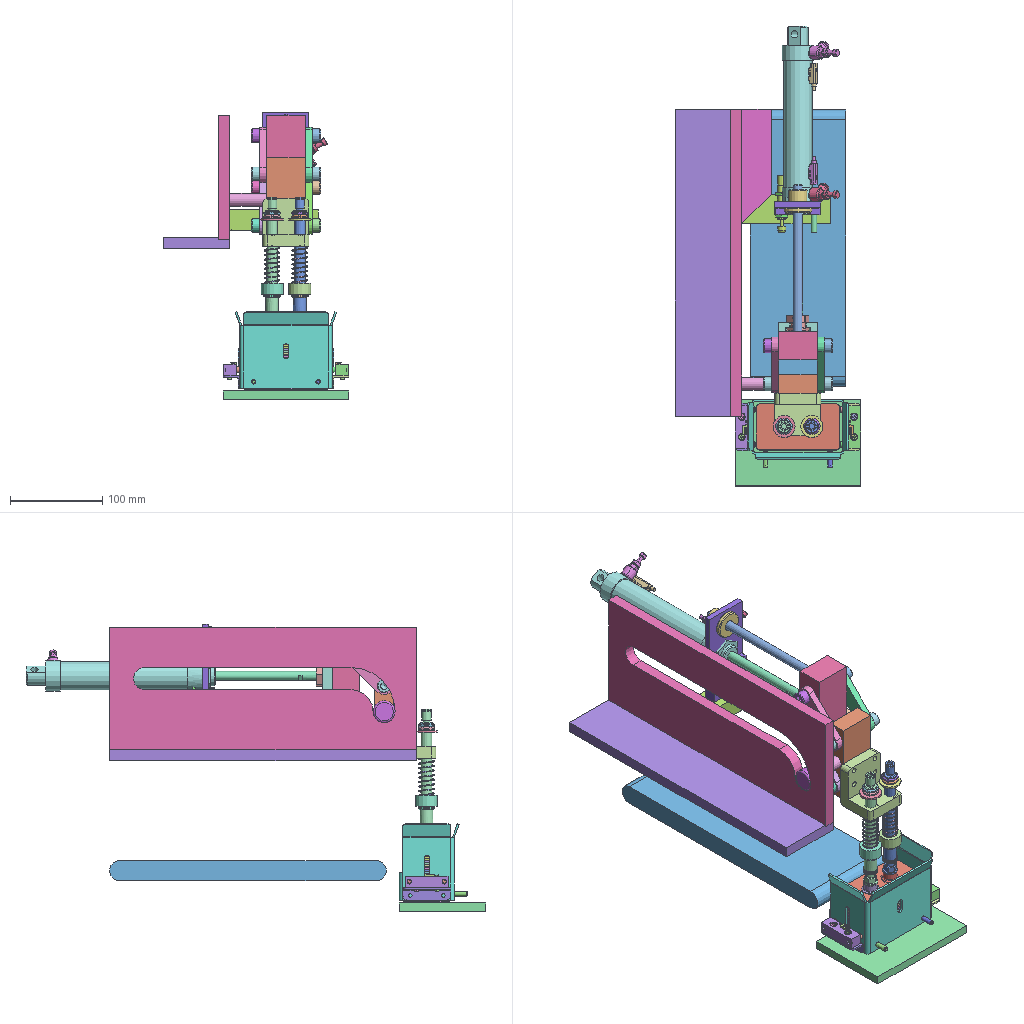Assembly | NX | 102 different items | 102 placed | box 201 x 499 x 312 mm
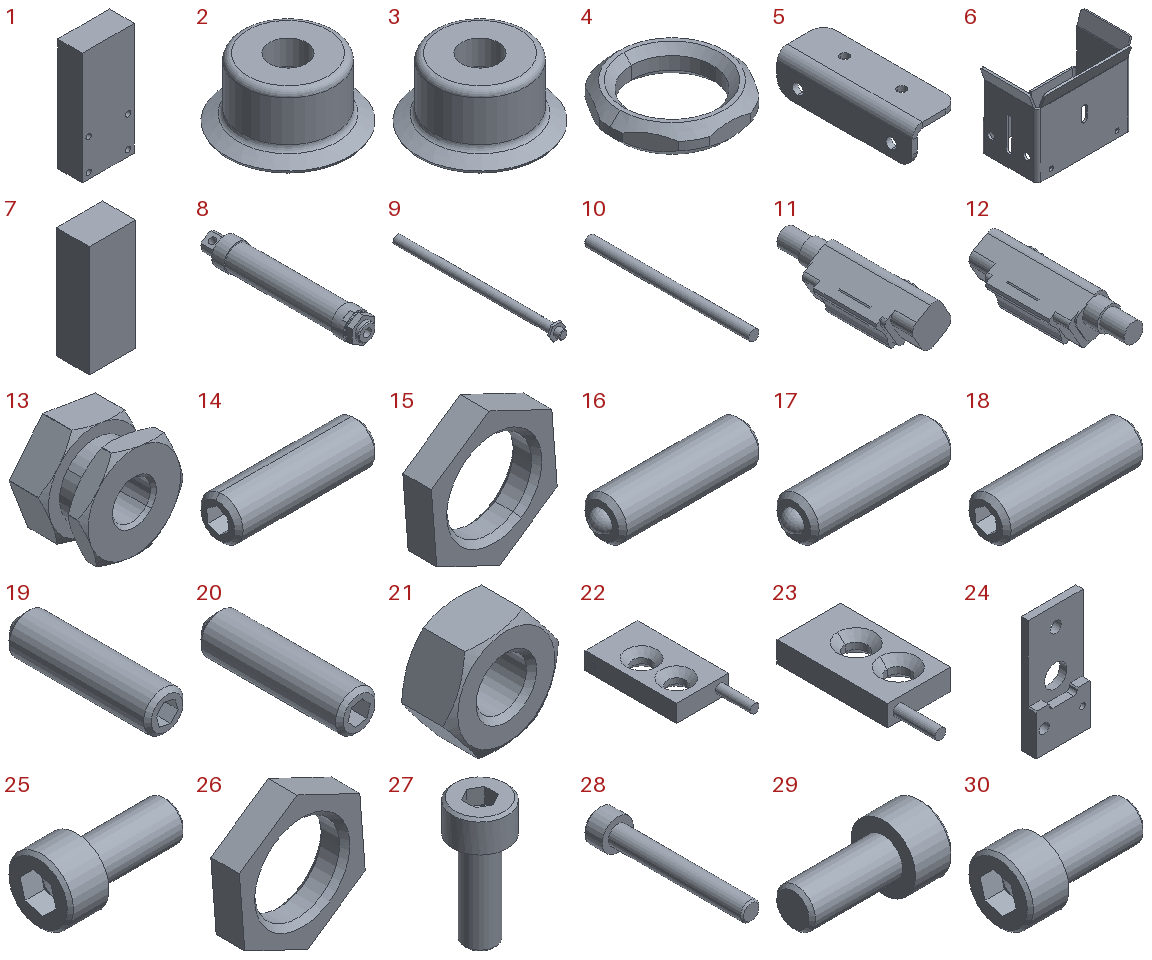Parts list (item | quantity | size | volume | features):
1 | x1 | 42 x 20 x 91 mm | 75332 mm3 | features M5 螺纹孔1 2
2 | x1 | 20 x 20 x 10 mm | 1200 mm3 | features 输入1 2
3 | x1 | 20 x 20 x 10 mm | 1200 mm3 | features 输入1 2
4 | x1 | 18 x 17 x 4 mm | 405.702 mm3 | features 输入1 2
5 | x1 | 18 x 52 x 14 mm | 2859 mm3 | features 镜向1 2
6 | x1 | 110.019 x 65.01 x 82.801 mm | 38324 mm3 | features M5 螺纹孔1 2
7 | x1 | 42 x 30 x 101 mm | 127260 mm3 | features M5 螺纹孔1 2
8 | x1 | 34 x 205 x 34 mm | 131750 mm3 | features WGN01-25-100-Y-2-001 2
9 | x1 | 19.589 x 203 x 17.595 mm | 16333 mm3 | features WGN01-25-100-Y-2-002 2
10 | x1 | 10 x 159.55 x 10 mm | 12516 mm3 | features WGN01-25-100-Y-2-002 2
11 | x1 | 10.179 x 30 x 9.481 mm | 1272 mm3 | features WGN01-25-100-Y-2-003 2
12 | x1 | 10.179 x 30 x 9.481 mm | 1272 mm3 | features WGN01-25-100-Y-2-003 2
13 | x1 | 23.903 x 16.5 x 22.65 mm | 4391 mm3 | features WHC31-M10-1_25-L8.SLDPRT 2
14 | x1 | 21.3 x 6 x 6 mm | 545.053 mm3 | features _ZAH01-M6 2
15 | x1 | 13.228 x 3 x 14.621 mm | 223.149 mm3 | features CONE_1 2
16 | x1 | 21.3 x 6 x 6 mm | 545.05 mm3 | features _ZAH01-M6 2
17 | x1 | 21.3 x 6 x 6 mm | 545.05 mm3 | features _ZAH01-M6 2
18 | x1 | 21.3 x 6 x 6 mm | 545.05 mm3 | features _ZAH01-M6 2
19 | x1 | 5 x 19.3 x 5 mm | 344.732 mm3 | features _ZAH04-M5 2
20 | x1 | 5 x 19.3 x 5 mm | 344.732 mm3 | features _ZAH04-M5 2
21 | x1 | 11.434 x 5.2 x 10.707 mm | 339.24 mm3 | features 倒角1 2
22 | x1 | 6.1 x 14.5 x 2 mm | 107.405 mm3 | features 倒角1 2
23 | x1 | 6.1 x 14.5 x 2 mm | 107.405 mm3 | features 倒角1 2
24 | x1 | 50 x 13.5 x 106 mm | 42427 mm3 | features 倒角2 2
25 | x1 | 30 x 15 x 15 mm | 2656 mm3 | features 切除-拉伸1 2
26 | x1 | 13.228 x 3 x 14.621 mm | 223.149 mm3 | features CONE_1 2
27 | x1 | 7 x 7 x 16 mm | 285.405 mm3 | features 切除-拉伸1 2
28 | x1 | 10 x 49 x 10 mm | 1607 mm3 | features 切除-拉伸1 2
29 | x1 | 30 x 15 x 15 mm | 2656 mm3 | features 切除-拉伸1 2
30 | x1 | 30 x 15 x 15 mm | 2656 mm3 | features 切除-拉伸1 2
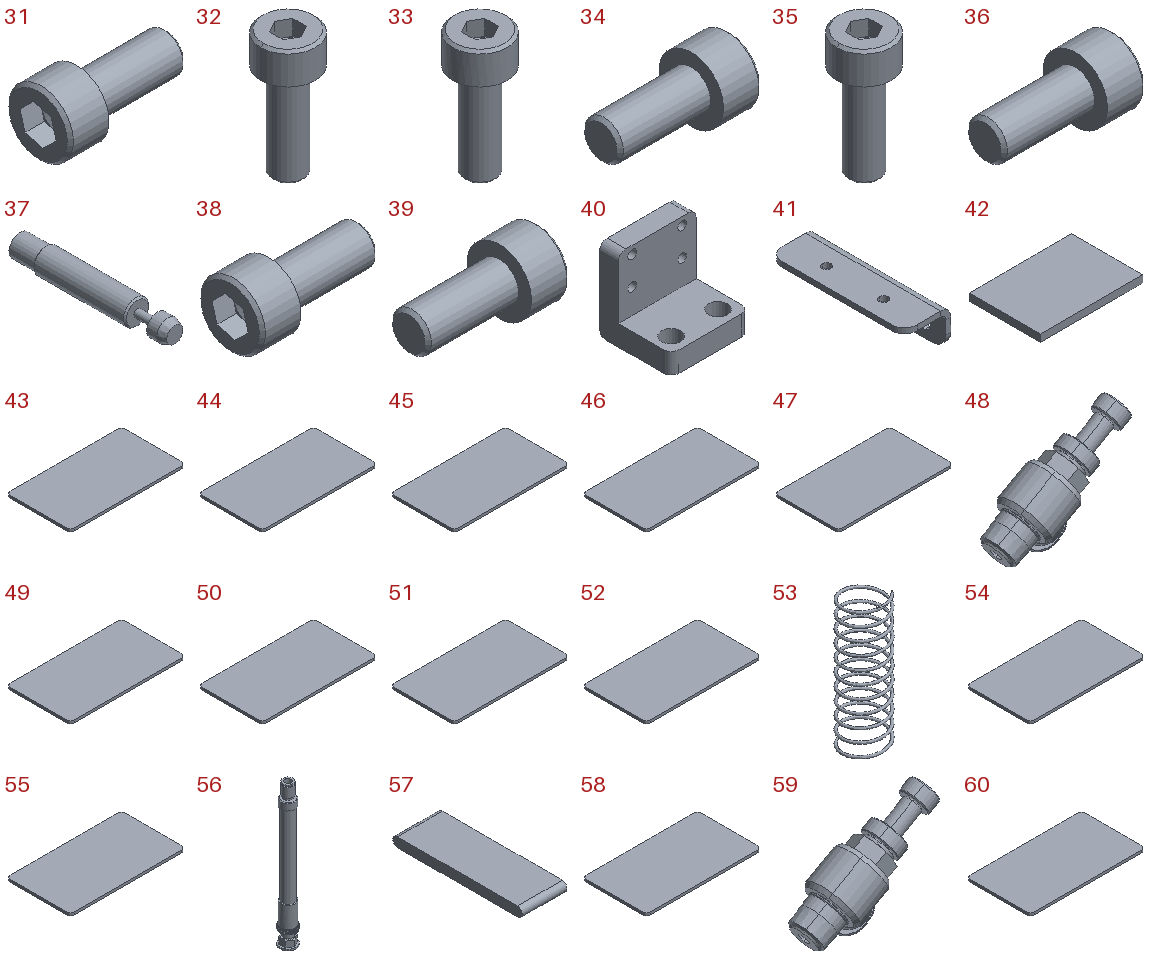31 | x1 | 30 x 15 x 15 mm | 2656 mm3 | features 切除-拉伸1 2
32 | x1 | 7 x 7 x 16 mm | 285.405 mm3 | features 切除-拉伸1 2
33 | x1 | 7 x 7 x 16 mm | 285.405 mm3 | features 切除-拉伸1 2
34 | x1 | 30 x 15 x 15 mm | 2656 mm3 | features 切除-拉伸1 2
35 | x1 | 7 x 7 x 16 mm | 285.405 mm3 | features 切除-拉伸1 2
36 | x1 | 30 x 15 x 15 mm | 2656 mm3 | features 切除-拉伸1 2
37 | x1 | 10 x 62 x 10 mm | 3924 mm3 | features CYL_3 2
38 | x1 | 30 x 15 x 15 mm | 2656 mm3 | features 切除-拉伸1 2
39 | x1 | 30 x 15 x 15 mm | 2656 mm3 | features 切除-拉伸1 2
40 | x1 | 50 x 46 x 52 mm | 48680 mm3 | features 切除-拉伸3 2
41 | x1 | 18 x 52 x 14 mm | 2859 mm3 | features 切除-拉伸4 2
42 | x1 | 136 x 94 x 9.5 mm | 121448 mm3 | features 打孔尺寸(%根据)内六角圆柱头螺钉的类型1 2
43 | x1 | 90 x 50 x 2 mm | 8985 mm3 | features solid 2
44 | x1 | 90 x 50 x 2 mm | 8985 mm3 | features solid 2
45 | x1 | 90 x 50 x 2 mm | 8985 mm3 | features solid 2
46 | x1 | 90 x 50 x 2 mm | 8985 mm3 | features solid 2
47 | x1 | 90 x 50 x 2 mm | 8985 mm3 | features solid 2
48 | x1 | 39.672 x 19.542 x 34.537 mm | 4093 mm3 | features J-XZB01-D6-1.SLDPRT 2
49 | x1 | 90 x 50 x 2 mm | 8985 mm3 | features solid 2
50 | x1 | 90 x 50 x 2 mm | 8985 mm3 | features solid 2
51 | x1 | 90 x 50 x 2 mm | 8985 mm3 | features solid 2
52 | x1 | 90 x 50 x 2 mm | 8985 mm3 | features solid 2
53 | x1 | 17.001 x 17.001 x 52 mm | 425.076 mm3 | features solid 2
54 | x1 | 90 x 50 x 2 mm | 8985 mm3 | features solid 2
55 | x1 | 90 x 50 x 2 mm | 8985 mm3 | features solid 2
56 | x1 | 16 x 16.9 x 142.1 mm | 16500 mm3 | features solid 2
57 | x1 | 104 x 300.3 x 22 mm | 676284 mm3 | features solid 2
58 | x1 | 90 x 50 x 2 mm | 8985 mm3 | features solid 2
59 | x1 | 39.672 x 19.542 x 34.537 mm | 4093 mm3 | features J-XZB01-D6-1.SLDPRT 2
60 | x1 | 90 x 50 x 2 mm | 8985 mm3 | features solid 2
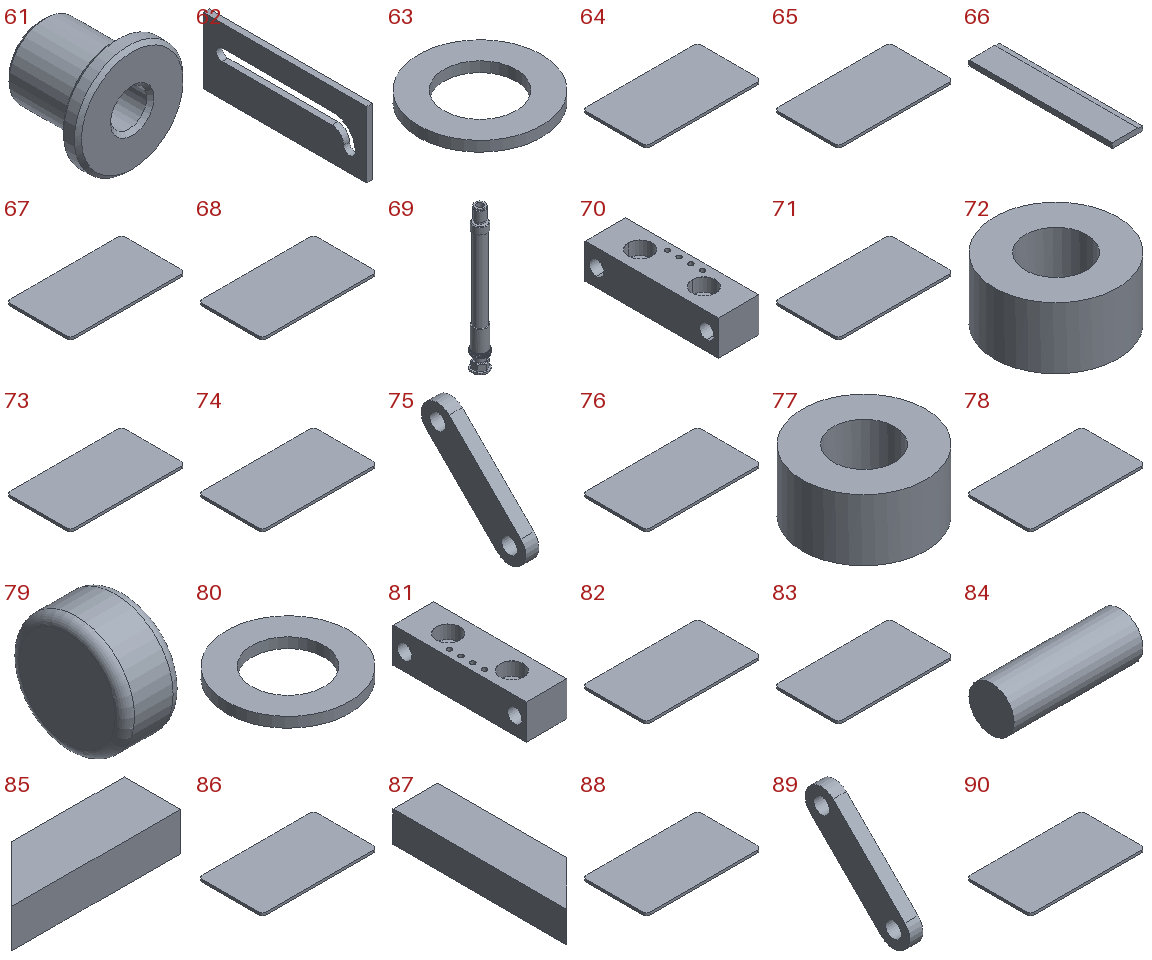61 | x1 | 30 x 25 x 30 mm | 7715 mm3 | features solid 2
62 | x1 | 12 x 333 x 135 mm | 453234 mm3 | features solid 2
63 | x1 | 24 x 24 x 2 mm | 596.903 mm3 | features solid 2
64 | x1 | 90 x 50 x 2 mm | 8985 mm3 | features solid 2
65 | x1 | 90 x 50 x 2 mm | 8985 mm3 | features solid 2
66 | x1 | 72 x 333 x 12 mm | 279720 mm3 | features solid 2
67 | x1 | 90 x 50 x 2 mm | 8985 mm3 | features solid 2
68 | x1 | 90 x 50 x 2 mm | 8985 mm3 | features solid 2
69 | x1 | 16 x 16.9 x 142.1 mm | 16500 mm3 | features solid 2
70 | x1 | 14 x 46 x 12 mm | 6437 mm3 | features M2 螺纹孔1 2
71 | x1 | 90 x 50 x 2 mm | 8985 mm3 | features solid 2
72 | x1 | 24 x 24 x 12 mm | 4072 mm3 | features solid 2
73 | x1 | 90 x 50 x 2 mm | 8985 mm3 | features solid 2
74 | x1 | 90 x 50 x 2 mm | 8985 mm3 | features solid 2
75 | x1 | 7.5 x 60.366 x 60.366 mm | 9508 mm3 | features solid 2
76 | x1 | 90 x 50 x 2 mm | 8985 mm3 | features solid 2
77 | x1 | 24 x 24 x 12 mm | 4072 mm3 | features solid 2
78 | x1 | 90 x 50 x 2 mm | 8985 mm3 | features solid 2
79 | x1 | 12 x 24 x 24 mm | 5304 mm3 | features solid 2
80 | x1 | 24 x 24 x 2 mm | 596.903 mm3 | features solid 2
81 | x1 | 14 x 46 x 12 mm | 6437 mm3 | features M2 螺纹孔1 2
82 | x1 | 90 x 50 x 2 mm | 8985 mm3 | features solid 2
83 | x1 | 90 x 50 x 2 mm | 8985 mm3 | features solid 2
84 | x1 | 40 x 14 x 14 mm | 6158 mm3 | features solid 2
85 | x1 | 96 x 32 x 22 mm | 26641 mm3 | features solid 2
86 | x1 | 90 x 50 x 2 mm | 8985 mm3 | features solid 2
87 | x1 | 32 x 124.084 x 22 mm | 35993 mm3 | features solid 2
88 | x1 | 90 x 50 x 2 mm | 8985 mm3 | features solid 2
89 | x1 | 7.5 x 60.366 x 60.366 mm | 9508 mm3 | features solid 2
90 | x1 | 90 x 50 x 2 mm | 8985 mm3 | features solid 2
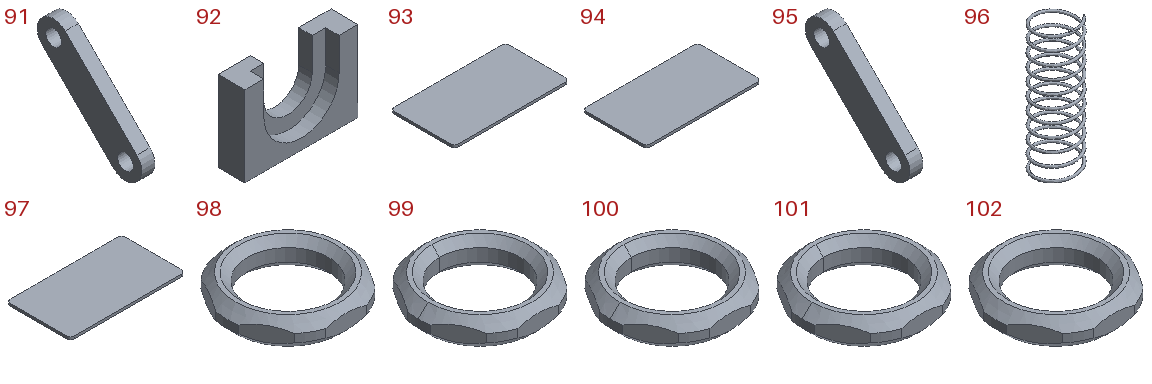91 | x1 | 7.5 x 60.366 x 60.366 mm | 9508 mm3 | features solid 2
92 | x1 | 42 x 10 x 30 mm | 7664 mm3 | features M5 六角凹头螺钉的柱形沉头孔1 2
93 | x1 | 90 x 50 x 2 mm | 8985 mm3 | features solid 2
94 | x1 | 90 x 50 x 2 mm | 8985 mm3 | features solid 2
95 | x1 | 7.5 x 60.366 x 60.366 mm | 9508 mm3 | features solid 2
96 | x1 | 17.001 x 17.001 x 52 mm | 425.076 mm3 | features solid 2
97 | x1 | 90 x 50 x 2 mm | 8985 mm3 | features solid 2
98 | x1 | 18 x 17 x 4 mm | 405.702 mm3 | features 输入1 2
99 | x1 | 18 x 17 x 4 mm | 405.702 mm3 | features 输入1 2
100 | x1 | 18 x 17 x 4 mm | 405.702 mm3 | features 输入1 2
101 | x1 | 18 x 17 x 4 mm | 405.702 mm3 | features 输入1 2
102 | x1 | 18 x 17 x 4 mm | 405.702 mm3 | features 输入1 2